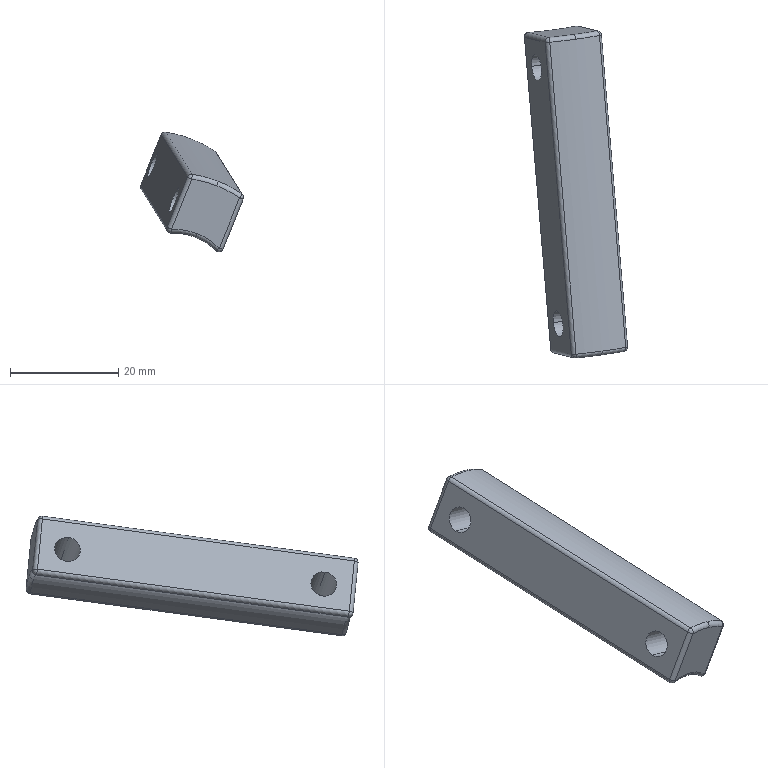Part | SolidWorks | features SplitBody 1 | 1 solid | 38 faces | box 19.087 x 61.426 x 22.135 mm | volume 7223 mm3 | cylinder 16 | sphere 10 | torus 8 | plane 4 | commonest cylinder face diameters 1.6 x10 4.8 x4 22.4 x1 44.8 x1
STEP:
#1=CARTESIAN_POINT('',(555.469,342.028,-348.256));
#2=VERTEX_POINT('',#1);
#3=CARTESIAN_POINT('',(554.431,342.001,-348.705));
#4=VERTEX_POINT('',#3);
#5=CARTESIAN_POINT('',(554.73,341.927,-347.967));
#6=DIRECTION('',(-0.08315,0.9876,0.1332));
#7=DIRECTION('',(-0.374,0.09296,-0.9228));
#8=AXIS2_PLACEMENT_3D('',#5,#6,#7);
#9=CIRCLE('',#8,0.8);
#10=EDGE_CURVE('',#2,#4,#9,.T.);
#11=ORIENTED_EDGE('',*,*,#10,.T.);
#12=CARTESIAN_POINT('',(554.663,342.717,-347.86));
#13=VERTEX_POINT('',#12);
#14=CARTESIAN_POINT('',(554.73,341.927,-347.967));
#15=DIRECTION('',(0.9237,0.1265,-0.3616));
#16=DIRECTION('',(-0.3646,0.,-0.9312));
#17=AXIS2_PLACEMENT_3D('',#14,#15,#16);
#18=CIRCLE('',#17,0.8);
#19=EDGE_CURVE('',#4,#13,#18,.T.);
#20=ORIENTED_EDGE('',*,*,#19,.T.);
#21=CARTESIAN_POINT('',(554.73,341.927,-347.967));
#22=DIRECTION('',(0.374,-0.09296,0.9228));
#23=DIRECTION('',(0.9237,0.1265,-0.3616));
#24=AXIS2_PLACEMENT_3D('',#21,#22,#23);
#25=CIRCLE('',#24,0.8);
#26=EDGE_CURVE('',#2,#13,#25,.T.);
#27=ORIENTED_EDGE('',*,*,#26,.F.);
#28=EDGE_LOOP('',(#11,#20,#27));
#29=FACE_OUTER_BOUND('',#28,.T.);
#30=CARTESIAN_POINT('',(554.73,341.927,-347.967));
#31=DIRECTION('',(-0.9237,-0.1265,0.3616));
#32=DIRECTION('',(-0.374,0.09296,-0.9228));
#33=AXIS2_PLACEMENT_3D('',#30,#31,#32);
#34=SPHERICAL_SURFACE('',#33,0.8);
#35=ADVANCED_FACE('',(#29),#34,.T.);
#36=CARTESIAN_POINT('',(554.195,341.124,-336.341));
#37=VERTEX_POINT('',#36);
#38=CARTESIAN_POINT('',(558.427,341.781,-338.576));
#39=VERTEX_POINT('',#38);
#40=CARTESIAN_POINT('',(546.116,343.132,-356.273));
#41=DIRECTION('',(-0.08315,0.9876,0.1332));
#42=DIRECTION('',(0.374,-0.09296,0.9228));
#43=AXIS2_PLACEMENT_3D('',#40,#41,#42);
#44=CIRCLE('',#43,21.6);
#45=EDGE_CURVE('',#37,#39,#44,.T.);
#46=ORIENTED_EDGE('',*,*,#45,.F.);
#47=CARTESIAN_POINT('',(554.561,340.259,-335.71));
#48=VERTEX_POINT('',#47);
#49=CARTESIAN_POINT('',(554.261,340.334,-336.448));
#50=DIRECTION('',(0.9237,0.1265,-0.3616));
#51=DIRECTION('',(-0.3646,0.,-0.9312));
#52=AXIS2_PLACEMENT_3D('',#49,#50,#51);
#53=CIRCLE('',#52,0.8);
#54=EDGE_CURVE('',#37,#48,#53,.T.);
#55=ORIENTED_EDGE('',*,*,#54,.T.);
#56=CARTESIAN_POINT('',(558.949,340.941,-338.027));
#57=VERTEX_POINT('',#56);
#58=CARTESIAN_POINT('',(546.183,342.342,-356.379));
#59=DIRECTION('',(0.08315,-0.9876,-0.1332));
#60=DIRECTION('',(0.374,-0.09296,0.9228));
#61=AXIS2_PLACEMENT_3D('',#58,#59,#60);
#62=CIRCLE('',#61,22.4);
#63=EDGE_CURVE('',#57,#48,#62,.T.);
#64=ORIENTED_EDGE('',*,*,#63,.F.);
#65=CARTESIAN_POINT('',(558.493,340.991,-338.682));
#66=DIRECTION('',(0.8175,0.144,-0.5577));
#67=DIRECTION('',(0.5699,-0.06252,0.8193));
#68=AXIS2_PLACEMENT_3D('',#65,#66,#67);
#69=CIRCLE('',#68,0.8);
#70=EDGE_CURVE('',#39,#57,#69,.T.);
#71=ORIENTED_EDGE('',*,*,#70,.F.);
#72=EDGE_LOOP('',(#46,#55,#64,#71));
#73=FACE_OUTER_BOUND('',#72,.T.);
#74=CARTESIAN_POINT('',(546.183,342.342,-356.379));
#75=DIRECTION('',(0.08315,-0.9876,-0.1332));
#76=DIRECTION('',(0.374,-0.09296,0.9228));
#77=AXIS2_PLACEMENT_3D('',#74,#75,#76);
#78=TOROIDAL_SURFACE('',#77,21.6,0.8);
#79=ADVANCED_FACE('',(#73),#78,.T.);
#80=CARTESIAN_POINT('',(560.325,284.352,-356.035));
#81=VERTEX_POINT('',#80);
#82=CARTESIAN_POINT('',(559.287,284.325,-356.484));
#83=VERTEX_POINT('',#82);
#84=CARTESIAN_POINT('',(559.586,284.251,-355.745));
#85=DIRECTION('',(-0.08315,0.9876,0.1332));
#86=DIRECTION('',(0.374,-0.09296,0.9228));
#87=AXIS2_PLACEMENT_3D('',#84,#85,#86);
#88=CIRCLE('',#87,0.8);
#89=EDGE_CURVE('',#81,#83,#88,.T.);
#90=ORIENTED_EDGE('',*,*,#89,.T.);
#91=CARTESIAN_POINT('',(559.353,283.535,-356.59));
#92=DIRECTION('',(-0.08315,0.9876,0.1332));
#93=VECTOR('',#92,1000.);
#94=LINE('',#91,#93);
#95=EDGE_CURVE('',#83,#4,#94,.T.);
#96=ORIENTED_EDGE('',*,*,#95,.T.);
#97=ORIENTED_EDGE('',*,*,#10,.F.);
#98=CARTESIAN_POINT('',(560.391,283.562,-356.141));
#99=DIRECTION('',(-0.08315,0.9876,0.1332));
#100=VECTOR('',#99,1000.);
#101=LINE('',#98,#100);
#102=EDGE_CURVE('',#81,#2,#101,.T.);
#103=ORIENTED_EDGE('',*,*,#102,.F.);
#104=EDGE_LOOP('',(#90,#96,#97,#103));
#105=FACE_OUTER_BOUND('',#104,.T.);
#106=CARTESIAN_POINT('',(559.653,283.461,-355.852));
#107=DIRECTION('',(-0.08315,0.9876,0.1332));
#108=DIRECTION('',(-0.374,0.09296,-0.9228));
#109=AXIS2_PLACEMENT_3D('',#106,#107,#108);
#110=CYLINDRICAL_SURFACE('',#109,0.8);
#111=ADVANCED_FACE('',(#105),#110,.T.);
#112=CARTESIAN_POINT('',(550.372,341.3,-346.044));
#113=VERTEX_POINT('',#112);
#114=CARTESIAN_POINT('',(554.16,341.954,-348.527));
#115=VERTEX_POINT('',#114);
#116=CARTESIAN_POINT('',(546.183,342.342,-356.379));
#117=DIRECTION('',(-0.08315,0.9876,0.1332));
#118=DIRECTION('',(0.374,-0.09296,0.9228));
#119=AXIS2_PLACEMENT_3D('',#116,#117,#118);
#120=CIRCLE('',#119,11.2);
#121=EDGE_CURVE('',#113,#115,#120,.T.);
#122=ORIENTED_EDGE('',*,*,#121,.F.);
#123=CARTESIAN_POINT('',(550.604,342.016,-345.2));
#124=VERTEX_POINT('',#123);
#125=CARTESIAN_POINT('',(550.671,341.226,-345.306));
#126=DIRECTION('',(0.9237,0.1265,-0.3616));
#127=DIRECTION('',(-0.3646,0.,-0.9312));
#128=AXIS2_PLACEMENT_3D('',#125,#126,#127);
#129=CIRCLE('',#128,0.8);
#130=EDGE_CURVE('',#113,#124,#129,.T.);
#131=ORIENTED_EDGE('',*,*,#130,.T.);
#132=CARTESIAN_POINT('',(546.116,343.132,-356.273));
#133=DIRECTION('',(0.08315,-0.9876,-0.1332));
#134=DIRECTION('',(0.374,-0.09296,0.9228));
#135=AXIS2_PLACEMENT_3D('',#132,#133,#134);
#136=CIRCLE('',#135,12.);
#137=EDGE_CURVE('',#13,#124,#136,.T.);
#138=ORIENTED_EDGE('',*,*,#137,.F.);
#139=CARTESIAN_POINT('',(554.73,341.927,-347.967));
#140=DIRECTION('',(0.697,0.1532,-0.7006));
#141=DIRECTION('',(0.7123,-0.03458,0.7011));
#142=AXIS2_PLACEMENT_3D('',#139,#140,#141);
#143=CIRCLE('',#142,0.8);
#144=EDGE_CURVE('',#115,#13,#143,.T.);
#145=ORIENTED_EDGE('',*,*,#144,.F.);
#146=EDGE_LOOP('',(#122,#131,#138,#145));
#147=FACE_OUTER_BOUND('',#146,.T.);
#148=CARTESIAN_POINT('',(546.183,342.342,-356.379));
#149=DIRECTION('',(0.08315,-0.9876,-0.1332));
#150=DIRECTION('',(0.374,-0.09296,0.9228));
#151=AXIS2_PLACEMENT_3D('',#148,#149,#150);
#152=TOROIDAL_SURFACE('',#151,12.,0.8);
#153=ADVANCED_FACE('',(#147),#152,.T.);
#154=CARTESIAN_POINT('',(545.884,340.82,-345.287));
#155=VERTEX_POINT('',#154);
#156=CARTESIAN_POINT('',(545.563,340.786,-345.233));
#157=VERTEX_POINT('',#156);
#158=CARTESIAN_POINT('',(545.863,340.712,-344.495));
#159=DIRECTION('',(-0.08315,0.9876,0.1332));
#160=DIRECTION('',(-0.374,0.09296,-0.9228));
#161=AXIS2_PLACEMENT_3D('',#158,#159,#160);
#162=CIRCLE('',#161,0.8);
#163=EDGE_CURVE('',#155,#157,#162,.T.);
#164=ORIENTED_EDGE('',*,*,#163,.T.);
#165=CARTESIAN_POINT('',(545.796,341.502,-344.388));
#166=VERTEX_POINT('',#165);
#167=CARTESIAN_POINT('',(545.863,340.712,-344.495));
#168=DIRECTION('',(0.9237,0.1265,-0.3616));
#169=DIRECTION('',(-0.3646,0.,-0.9312));
#170=AXIS2_PLACEMENT_3D('',#167,#168,#169);
#171=CIRCLE('',#170,0.8);
#172=EDGE_CURVE('',#157,#166,#171,.T.);
#173=ORIENTED_EDGE('',*,*,#172,.T.);
#174=CARTESIAN_POINT('',(545.863,340.712,-344.495));
#175=DIRECTION('',(0.9962,0.0788,0.03765));
#176=DIRECTION('',(0.02668,0.1358,-0.9904));
#177=AXIS2_PLACEMENT_3D('',#174,#175,#176);
#178=CIRCLE('',#177,0.8);
#179=EDGE_CURVE('',#155,#166,#178,.T.);
#180=ORIENTED_EDGE('',*,*,#179,.F.);
#181=EDGE_LOOP('',(#164,#173,#180));
#182=FACE_OUTER_BOUND('',#181,.T.);
#183=CARTESIAN_POINT('',(545.863,340.712,-344.495));
#184=DIRECTION('',(-0.9237,-0.1265,0.3616));
#185=DIRECTION('',(-0.374,0.09296,-0.9228));
#186=AXIS2_PLACEMENT_3D('',#183,#184,#185);
#187=SPHERICAL_SURFACE('',#186,0.8);
#188=ADVANCED_FACE('',(#182),#187,.T.);
#189=CARTESIAN_POINT('',(559.417,282.584,-343.488));
#190=VERTEX_POINT('',#189);
#191=CARTESIAN_POINT('',(563.805,283.266,-345.805));
#192=VERTEX_POINT('',#191);
#193=CARTESIAN_POINT('',(551.039,284.666,-364.158));
#194=DIRECTION('',(-0.08315,0.9876,0.1332));
#195=DIRECTION('',(0.374,-0.09296,0.9228));
#196=AXIS2_PLACEMENT_3D('',#193,#194,#195);
#197=CIRCLE('',#196,22.4);
#198=EDGE_CURVE('',#190,#192,#197,.T.);
#199=ORIENTED_EDGE('',*,*,#198,.F.);
#200=CARTESIAN_POINT('',(559.184,281.868,-344.333));
#201=VERTEX_POINT('',#200);
#202=CARTESIAN_POINT('',(559.118,282.658,-344.227));
#203=DIRECTION('',(0.9237,0.1265,-0.3616));
#204=DIRECTION('',(-0.3646,0.,-0.9312));
#205=AXIS2_PLACEMENT_3D('',#202,#203,#204);
#206=CIRCLE('',#205,0.8);
#207=EDGE_CURVE('',#190,#201,#206,.T.);
#208=ORIENTED_EDGE('',*,*,#207,.T.);
#209=CARTESIAN_POINT('',(563.416,282.526,-346.567));
#210=VERTEX_POINT('',#209);
#211=CARTESIAN_POINT('',(551.105,283.876,-364.265));
#212=DIRECTION('',(0.08315,-0.9876,-0.1332));
#213=DIRECTION('',(0.374,-0.09296,0.9228));
#214=AXIS2_PLACEMENT_3D('',#211,#212,#213);
#215=CIRCLE('',#214,21.6);
#216=EDGE_CURVE('',#210,#201,#215,.T.);
#217=ORIENTED_EDGE('',*,*,#216,.F.);
#218=CARTESIAN_POINT('',(563.349,283.316,-346.461));
#219=DIRECTION('',(0.8175,0.144,-0.5577));
#220=DIRECTION('',(0.5699,-0.06252,0.8193));
#221=AXIS2_PLACEMENT_3D('',#218,#219,#220);
#222=CIRCLE('',#221,0.8);
#223=EDGE_CURVE('',#192,#210,#222,.T.);
#224=ORIENTED_EDGE('',*,*,#223,.F.);
#225=EDGE_LOOP('',(#199,#208,#217,#224));
#226=FACE_OUTER_BOUND('',#225,.T.);
#227=CARTESIAN_POINT('',(551.039,284.666,-364.158));
#228=DIRECTION('',(0.08315,-0.9876,-0.1332));
#229=DIRECTION('',(0.374,-0.09296,0.9228));
#230=AXIS2_PLACEMENT_3D('',#227,#228,#229);
#231=TOROIDAL_SURFACE('',#230,21.6,0.8);
#232=ADVANCED_FACE('',(#226),#231,.T.);
#233=CARTESIAN_POINT('',(555.594,282.76,-353.192));
#234=VERTEX_POINT('',#233);
#235=CARTESIAN_POINT('',(559.653,283.461,-355.852));
#236=VERTEX_POINT('',#235);
#237=CARTESIAN_POINT('',(551.105,283.876,-364.265));
#238=DIRECTION('',(-0.08315,0.9876,0.1332));
#239=DIRECTION('',(0.374,-0.09296,0.9228));
#240=AXIS2_PLACEMENT_3D('',#237,#238,#239);
#241=CIRCLE('',#240,12.);
#242=EDGE_CURVE('',#234,#236,#241,.T.);
#243=ORIENTED_EDGE('',*,*,#242,.F.);
#244=CARTESIAN_POINT('',(555.228,283.625,-353.823));
#245=VERTEX_POINT('',#244);
#246=CARTESIAN_POINT('',(555.527,283.551,-353.085));
#247=DIRECTION('',(0.9237,0.1265,-0.3616));
#248=DIRECTION('',(-0.3646,0.,-0.9312));
#249=AXIS2_PLACEMENT_3D('',#246,#247,#248);
#250=CIRCLE('',#249,0.8);
#251=EDGE_CURVE('',#234,#245,#250,.T.);
#252=ORIENTED_EDGE('',*,*,#251,.T.);
#253=CARTESIAN_POINT('',(559.016,284.279,-356.306));
#254=VERTEX_POINT('',#253);
#255=CARTESIAN_POINT('',(551.039,284.666,-364.158));
#256=DIRECTION('',(0.08315,-0.9876,-0.1332));
#257=DIRECTION('',(0.374,-0.09296,0.9228));
#258=AXIS2_PLACEMENT_3D('',#255,#256,#257);
#259=CIRCLE('',#258,11.2);
#260=EDGE_CURVE('',#254,#245,#259,.T.);
#261=ORIENTED_EDGE('',*,*,#260,.F.);
#262=CARTESIAN_POINT('',(559.586,284.251,-355.745));
#263=DIRECTION('',(0.697,0.1532,-0.7006));
#264=DIRECTION('',(0.7123,-0.03458,0.7011));
#265=AXIS2_PLACEMENT_3D('',#262,#263,#264);
#266=CIRCLE('',#265,0.8);
#267=EDGE_CURVE('',#236,#254,#266,.T.);
#268=ORIENTED_EDGE('',*,*,#267,.F.);
#269=EDGE_LOOP('',(#243,#252,#261,#268));
#270=FACE_OUTER_BOUND('',#269,.T.);
#271=CARTESIAN_POINT('',(551.039,284.666,-364.158));
#272=DIRECTION('',(0.08315,-0.9876,-0.1332));
#273=DIRECTION('',(0.374,-0.09296,0.9228));
#274=AXIS2_PLACEMENT_3D('',#271,#272,#273);
#275=TOROIDAL_SURFACE('',#274,12.,0.8);
#276=ADVANCED_FACE('',(#270),#275,.T.);
#277=CARTESIAN_POINT('',(550.74,283.145,-353.066));
#278=VERTEX_POINT('',#277);
#279=CARTESIAN_POINT('',(550.419,283.111,-353.012));
#280=VERTEX_POINT('',#279);
#281=CARTESIAN_POINT('',(550.719,283.036,-352.274));
#282=DIRECTION('',(-0.08315,0.9876,0.1332));
#283=DIRECTION('',(0.374,-0.09296,0.9228));
#284=AXIS2_PLACEMENT_3D('',#281,#282,#283);
#285=CIRCLE('',#284,0.8);
#286=EDGE_CURVE('',#278,#280,#285,.T.);
#287=ORIENTED_EDGE('',*,*,#286,.T.);
#288=CARTESIAN_POINT('',(550.486,282.321,-353.118));
#289=DIRECTION('',(-0.08315,0.9876,0.1332));
#290=VECTOR('',#289,1000.);
#291=LINE('',#288,#290);
#292=EDGE_CURVE('',#280,#157,#291,.T.);
#293=ORIENTED_EDGE('',*,*,#292,.T.);
#294=ORIENTED_EDGE('',*,*,#163,.F.);
#295=CARTESIAN_POINT('',(550.806,282.355,-353.172));
#296=DIRECTION('',(-0.08315,0.9876,0.1332));
#297=VECTOR('',#296,1000.);
#298=LINE('',#295,#297);
#299=EDGE_CURVE('',#278,#155,#298,.T.);
#300=ORIENTED_EDGE('',*,*,#299,.F.);
#301=EDGE_LOOP('',(#287,#293,#294,#300));
#302=FACE_OUTER_BOUND('',#301,.T.);
#303=CARTESIAN_POINT('',(550.785,282.246,-352.38));
#304=DIRECTION('',(-0.08315,0.9876,0.1332));
#305=DIRECTION('',(-0.374,0.09296,-0.9228));
#306=AXIS2_PLACEMENT_3D('',#303,#304,#305);
#307=CYLINDRICAL_SURFACE('',#306,0.8);
#308=ADVANCED_FACE('',(#302),#307,.T.);
#309=CARTESIAN_POINT('',(562.547,288.828,-348.794));
#310=VERTEX_POINT('',#309);
#311=CARTESIAN_POINT('',(560.751,289.274,-353.224));
#312=VERTEX_POINT('',#311);
#313=CARTESIAN_POINT('',(561.649,289.051,-351.009));
#314=DIRECTION('',(-0.9237,-0.1265,0.3616));
#315=DIRECTION('',(-0.374,0.09296,-0.9228));
#316=AXIS2_PLACEMENT_3D('',#313,#314,#315);
#317=CIRCLE('',#316,2.4);
#318=EDGE_CURVE('',#310,#312,#317,.T.);
#319=ORIENTED_EDGE('',*,*,#318,.F.);
#320=CARTESIAN_POINT('',(552.201,287.411,-344.744));
#321=VERTEX_POINT('',#320);
#322=CARTESIAN_POINT('',(562.547,288.828,-348.794));
#323=DIRECTION('',(-0.9237,-0.1265,0.3616));
#324=VECTOR('',#323,1000.);
#325=LINE('',#322,#324);
#326=EDGE_CURVE('',#310,#321,#325,.T.);
#327=ORIENTED_EDGE('',*,*,#326,.T.);
#328=CARTESIAN_POINT('',(550.406,287.857,-349.173));
#329=VERTEX_POINT('',#328);
#330=CARTESIAN_POINT('',(551.304,287.634,-346.958));
#331=DIRECTION('',(-0.9237,-0.1265,0.3616));
#332=DIRECTION('',(-0.374,0.09296,-0.9228));
#333=AXIS2_PLACEMENT_3D('',#330,#331,#332);
#334=CIRCLE('',#333,2.4);
#335=EDGE_CURVE('',#321,#329,#334,.T.);
#336=ORIENTED_EDGE('',*,*,#335,.T.);
#337=CARTESIAN_POINT('',(560.751,289.274,-353.224));
#338=DIRECTION('',(-0.9237,-0.1265,0.3616));
#339=VECTOR('',#338,1000.);
#340=LINE('',#337,#339);
#341=EDGE_CURVE('',#312,#329,#340,.T.);
#342=ORIENTED_EDGE('',*,*,#341,.F.);
#343=EDGE_LOOP('',(#319,#327,#336,#342));
#344=FACE_OUTER_BOUND('',#343,.T.);
#345=CARTESIAN_POINT('',(561.649,289.051,-351.009));
#346=DIRECTION('',(-0.9237,-0.1265,0.3616));
#347=DIRECTION('',(-0.374,0.09296,-0.9228));
#348=AXIS2_PLACEMENT_3D('',#345,#346,#347);
#349=CYLINDRICAL_SURFACE('',#348,2.4);
#350=ADVANCED_FACE('',(#344),#349,.F.);
#351=CARTESIAN_POINT('',(558.555,336.233,-342.401));
#352=VERTEX_POINT('',#351);
#353=CARTESIAN_POINT('',(556.76,336.679,-346.83));
#354=VERTEX_POINT('',#353);
#355=CARTESIAN_POINT('',(557.658,336.456,-344.615));
#356=DIRECTION('',(-0.9237,-0.1265,0.3616));
#357=DIRECTION('',(-0.374,0.09296,-0.9228));
#358=AXIS2_PLACEMENT_3D('',#355,#356,#357);
#359=CIRCLE('',#358,2.4);
#360=EDGE_CURVE('',#352,#354,#359,.T.);
#361=ORIENTED_EDGE('',*,*,#360,.F.);
#362=CARTESIAN_POINT('',(548.21,334.815,-338.35));
#363=VERTEX_POINT('',#362);
#364=CARTESIAN_POINT('',(558.555,336.233,-342.401));
#365=DIRECTION('',(-0.9237,-0.1265,0.3616));
#366=VECTOR('',#365,1000.);
#367=LINE('',#364,#366);
#368=EDGE_CURVE('',#352,#363,#367,.T.);
#369=ORIENTED_EDGE('',*,*,#368,.T.);
#370=CARTESIAN_POINT('',(546.415,335.262,-342.78));
#371=VERTEX_POINT('',#370);
#372=CARTESIAN_POINT('',(547.312,335.038,-340.565));
#373=DIRECTION('',(-0.9237,-0.1265,0.3616));
#374=DIRECTION('',(-0.374,0.09296,-0.9228));
#375=AXIS2_PLACEMENT_3D('',#372,#373,#374);
#376=CIRCLE('',#375,2.4);
#377=EDGE_CURVE('',#363,#371,#376,.T.);
#378=ORIENTED_EDGE('',*,*,#377,.T.);
#379=CARTESIAN_POINT('',(556.76,336.679,-346.83));
#380=DIRECTION('',(-0.9237,-0.1265,0.3616));
#381=VECTOR('',#380,1000.);
#382=LINE('',#379,#381);
#383=EDGE_CURVE('',#354,#371,#382,.T.);
#384=ORIENTED_EDGE('',*,*,#383,.F.);
#385=EDGE_LOOP('',(#361,#369,#378,#384));
#386=FACE_OUTER_BOUND('',#385,.T.);
#387=CARTESIAN_POINT('',(557.658,336.456,-344.615));
#388=DIRECTION('',(-0.9237,-0.1265,0.3616));
#389=DIRECTION('',(-0.374,0.09296,-0.9228));
#390=AXIS2_PLACEMENT_3D('',#387,#388,#389);
#391=CYLINDRICAL_SURFACE('',#390,2.4);
#392=ADVANCED_FACE('',(#386),#391,.F.);
#393=ORIENTED_EDGE('',*,*,#299,.T.);
#394=CARTESIAN_POINT('',(546.183,342.342,-356.379));
#395=DIRECTION('',(-0.08315,0.9876,0.1332));
#396=DIRECTION('',(0.374,-0.09296,0.9228));
#397=AXIS2_PLACEMENT_3D('',#394,#395,#396);
#398=CIRCLE('',#397,11.2);
#399=EDGE_CURVE('',#155,#113,#398,.T.);
#400=ORIENTED_EDGE('',*,*,#399,.T.);
#401=ORIENTED_EDGE('',*,*,#121,.T.);
#402=CARTESIAN_POINT('',(559.083,283.489,-356.413));
#403=DIRECTION('',(0.08315,-0.9876,-0.1332));
#404=VECTOR('',#403,1000.);
#405=LINE('',#402,#404);
#406=EDGE_CURVE('',#115,#254,#405,.T.);
#407=ORIENTED_EDGE('',*,*,#406,.T.);
#408=ORIENTED_EDGE('',*,*,#260,.T.);
#409=CARTESIAN_POINT('',(551.039,284.666,-364.158));
#410=DIRECTION('',(0.08315,-0.9876,-0.1332));
#411=DIRECTION('',(0.374,-0.09296,0.9228));
#412=AXIS2_PLACEMENT_3D('',#409,#410,#411);
#413=CIRCLE('',#412,11.2);
#414=EDGE_CURVE('',#245,#278,#413,.T.);
#415=ORIENTED_EDGE('',*,*,#414,.T.);
#416=EDGE_LOOP('',(#393,#400,#401,#407,#408,#415));
#417=FACE_OUTER_BOUND('',#416,.T.);
#418=CARTESIAN_POINT('',(551.105,283.876,-364.265));
#419=DIRECTION('',(-0.08315,0.9876,0.1332));
#420=DIRECTION('',(-0.374,0.09296,-0.9228));
#421=AXIS2_PLACEMENT_3D('',#418,#419,#420);
#422=CYLINDRICAL_SURFACE('',#421,11.2);
#423=ADVANCED_FACE('',(#417),#422,.F.);
#424=ORIENTED_EDGE('',*,*,#102,.T.);
#425=CARTESIAN_POINT('',(559.232,341.093,-338.971));
#426=VERTEX_POINT('',#425);
#427=CARTESIAN_POINT('',(554.983,342.149,-349.454));
#428=DIRECTION('',(0.374,-0.09296,0.9228));
#429=VECTOR('',#428,1000.);
#430=LINE('',#427,#429);
#431=EDGE_CURVE('',#2,#426,#430,.T.);
#432=ORIENTED_EDGE('',*,*,#431,.T.);
#433=CARTESIAN_POINT('',(564.088,283.417,-346.75));
#434=VERTEX_POINT('',#433);
#435=CARTESIAN_POINT('',(564.155,282.627,-346.857));
#436=DIRECTION('',(0.08315,-0.9876,-0.1332));
#437=VECTOR('',#436,1000.);
#438=LINE('',#435,#437);
#439=EDGE_CURVE('',#426,#434,#438,.T.);
#440=ORIENTED_EDGE('',*,*,#439,.T.);
#441=CARTESIAN_POINT('',(559.839,284.473,-357.233));
#442=DIRECTION('',(-0.374,0.09296,-0.9228));
#443=VECTOR('',#442,1000.);
#444=LINE('',#441,#443);
#445=EDGE_CURVE('',#434,#81,#444,.T.);
#446=ORIENTED_EDGE('',*,*,#445,.T.);
#447=EDGE_LOOP('',(#424,#432,#440,#446));
#448=FACE_OUTER_BOUND('',#447,.T.);
#449=CARTESIAN_POINT('',(561.649,289.051,-351.009));
#450=DIRECTION('',(-0.9237,-0.1265,0.3616));
#451=DIRECTION('',(-0.374,0.09296,-0.9228));
#452=AXIS2_PLACEMENT_3D('',#449,#450,#451);
#453=CIRCLE('',#452,2.4);
#454=EDGE_CURVE('',#312,#310,#453,.T.);
#455=ORIENTED_EDGE('',*,*,#454,.T.);
#456=ORIENTED_EDGE('',*,*,#318,.T.);
#457=EDGE_LOOP('',(#455,#456));
#458=FACE_BOUND('',#457,.T.);
#459=CARTESIAN_POINT('',(557.658,336.456,-344.615));
#460=DIRECTION('',(-0.9237,-0.1265,0.3616));
#461=DIRECTION('',(-0.374,0.09296,-0.9228));
#462=AXIS2_PLACEMENT_3D('',#459,#460,#461);
#463=CIRCLE('',#462,2.4);
#464=EDGE_CURVE('',#354,#352,#463,.T.);
#465=ORIENTED_EDGE('',*,*,#464,.T.);
#466=ORIENTED_EDGE('',*,*,#360,.T.);
#467=EDGE_LOOP('',(#465,#466));
#468=FACE_BOUND('',#467,.T.);
#469=CARTESIAN_POINT('',(559.906,283.683,-357.34));
#470=DIRECTION('',(-0.9237,-0.1265,0.3616));
#471=DIRECTION('',(-0.374,0.09296,-0.9228));
#472=AXIS2_PLACEMENT_3D('',#469,#470,#471);
#473=PLANE('',#472);
#474=ADVANCED_FACE('',(#448,#458,#468),#473,.F.);
#475=CARTESIAN_POINT('',(563.872,282.476,-345.912));
#476=DIRECTION('',(-0.08315,0.9876,0.1332));
#477=VECTOR('',#476,1000.);
#478=LINE('',#475,#477);
#479=EDGE_CURVE('',#192,#57,#478,.T.);
#480=ORIENTED_EDGE('',*,*,#479,.T.);
#481=ORIENTED_EDGE('',*,*,#63,.T.);
#482=CARTESIAN_POINT('',(549.753,339.681,-334.426));
#483=VERTEX_POINT('',#482);
#484=CARTESIAN_POINT('',(546.183,342.342,-356.379));
#485=DIRECTION('',(0.08315,-0.9876,-0.1332));
#486=DIRECTION('',(0.374,-0.09296,0.9228));
#487=AXIS2_PLACEMENT_3D('',#484,#485,#486);
#488=CIRCLE('',#487,22.4);
#489=EDGE_CURVE('',#48,#483,#488,.T.);
#490=ORIENTED_EDGE('',*,*,#489,.T.);
#491=CARTESIAN_POINT('',(554.609,282.006,-342.205));
#492=VERTEX_POINT('',#491);
#493=CARTESIAN_POINT('',(554.676,281.216,-342.312));
#494=DIRECTION('',(0.08315,-0.9876,-0.1332));
#495=VECTOR('',#494,1000.);
#496=LINE('',#493,#495);
#497=EDGE_CURVE('',#483,#492,#496,.T.);
#498=ORIENTED_EDGE('',*,*,#497,.T.);
#499=CARTESIAN_POINT('',(551.039,284.666,-364.158));
#500=DIRECTION('',(-0.08315,0.9876,0.1332));
#501=DIRECTION('',(0.374,-0.09296,0.9228));
#502=AXIS2_PLACEMENT_3D('',#499,#500,#501);
#503=CIRCLE('',#502,22.4);
#504=EDGE_CURVE('',#492,#190,#503,.T.);
#505=ORIENTED_EDGE('',*,*,#504,.T.);
#506=ORIENTED_EDGE('',*,*,#198,.T.);
#507=EDGE_LOOP('',(#480,#481,#490,#498,#505,#506));
#508=FACE_OUTER_BOUND('',#507,.T.);
#509=CARTESIAN_POINT('',(551.105,283.876,-364.265));
#510=DIRECTION('',(-0.08315,0.9876,0.1332));
#511=DIRECTION('',(-0.374,0.09296,-0.9228));
#512=AXIS2_PLACEMENT_3D('',#509,#510,#511);
#513=CYLINDRICAL_SURFACE('',#512,22.4);
#514=ADVANCED_FACE('',(#508),#513,.T.);
#515=CARTESIAN_POINT('',(553.743,282.,-342.7));
#516=VERTEX_POINT('',#515);
#517=CARTESIAN_POINT('',(548.887,339.675,-334.921));
#518=VERTEX_POINT('',#517);
#519=CARTESIAN_POINT('',(553.809,281.21,-342.806));
#520=DIRECTION('',(-0.08315,0.9876,0.1332));
#521=VECTOR('',#520,1000.);
#522=LINE('',#519,#521);
#523=EDGE_CURVE('',#516,#518,#522,.T.);
#524=ORIENTED_EDGE('',*,*,#523,.T.);
#525=CARTESIAN_POINT('',(545.124,340.611,-344.205));
#526=VERTEX_POINT('',#525);
#527=CARTESIAN_POINT('',(549.122,339.617,-334.341));
#528=DIRECTION('',(-0.374,0.09296,-0.9228));
#529=VECTOR('',#528,1000.);
#530=LINE('',#527,#529);
#531=EDGE_CURVE('',#518,#526,#530,.T.);
#532=ORIENTED_EDGE('',*,*,#531,.T.);
#533=CARTESIAN_POINT('',(549.98,282.935,-351.984));
#534=VERTEX_POINT('',#533);
#535=CARTESIAN_POINT('',(550.046,282.145,-352.091));
#536=DIRECTION('',(0.08315,-0.9876,-0.1332));
#537=VECTOR('',#536,1000.);
#538=LINE('',#535,#537);
#539=EDGE_CURVE('',#526,#534,#538,.T.);
#540=ORIENTED_EDGE('',*,*,#539,.T.);
#541=CARTESIAN_POINT('',(553.978,281.941,-342.12));
#542=DIRECTION('',(0.374,-0.09296,0.9228));
#543=VECTOR('',#542,1000.);
#544=LINE('',#541,#543);
#545=EDGE_CURVE('',#534,#516,#544,.T.);
#546=ORIENTED_EDGE('',*,*,#545,.T.);
#547=EDGE_LOOP('',(#524,#532,#540,#546));
#548=FACE_OUTER_BOUND('',#547,.T.);
#549=CARTESIAN_POINT('',(551.304,287.634,-346.958));
#550=DIRECTION('',(-0.9237,-0.1265,0.3616));
#551=DIRECTION('',(-0.374,0.09296,-0.9228));
#552=AXIS2_PLACEMENT_3D('',#549,#550,#551);
#553=CIRCLE('',#552,2.4);
#554=EDGE_CURVE('',#329,#321,#553,.T.);
#555=ORIENTED_EDGE('',*,*,#554,.F.);
#556=ORIENTED_EDGE('',*,*,#335,.F.);
#557=EDGE_LOOP('',(#555,#556));
#558=FACE_BOUND('',#557,.T.);
#559=CARTESIAN_POINT('',(547.312,335.038,-340.565));
#560=DIRECTION('',(-0.9237,-0.1265,0.3616));
#561=DIRECTION('',(-0.374,0.09296,-0.9228));
#562=AXIS2_PLACEMENT_3D('',#559,#560,#561);
#563=CIRCLE('',#562,2.4);
#564=EDGE_CURVE('',#371,#363,#563,.T.);
#565=ORIENTED_EDGE('',*,*,#564,.F.);
#566=ORIENTED_EDGE('',*,*,#377,.F.);
#567=EDGE_LOOP('',(#565,#566));
#568=FACE_BOUND('',#567,.T.);
#569=CARTESIAN_POINT('',(554.045,281.151,-342.226));
#570=DIRECTION('',(0.9237,0.1265,-0.3616));
#571=DIRECTION('',(0.374,-0.09296,0.9228));
#572=AXIS2_PLACEMENT_3D('',#569,#570,#571);
#573=PLANE('',#572);
#574=ADVANCED_FACE('',(#548,#558,#568),#573,.F.);
#575=ORIENTED_EDGE('',*,*,#216,.T.);
#576=CARTESIAN_POINT('',(554.548,281.311,-343.096));
#577=VERTEX_POINT('',#576);
#578=CARTESIAN_POINT('',(551.105,283.876,-364.265));
#579=DIRECTION('',(0.08315,-0.9876,-0.1332));
#580=DIRECTION('',(0.374,-0.09296,0.9228));
#581=AXIS2_PLACEMENT_3D('',#578,#579,#580);
#582=CIRCLE('',#581,21.6);
#583=EDGE_CURVE('',#201,#577,#582,.T.);
#584=ORIENTED_EDGE('',*,*,#583,.T.);
#585=CARTESIAN_POINT('',(550.785,282.246,-352.38));
#586=VERTEX_POINT('',#585);
#587=CARTESIAN_POINT('',(550.299,282.367,-353.579));
#588=DIRECTION('',(-0.374,0.09296,-0.9228));
#589=VECTOR('',#588,1000.);
#590=LINE('',#587,#589);
#591=EDGE_CURVE('',#577,#586,#590,.T.);
#592=ORIENTED_EDGE('',*,*,#591,.T.);
#593=CARTESIAN_POINT('',(551.105,283.876,-364.265));
#594=DIRECTION('',(-0.08315,0.9876,0.1332));
#595=DIRECTION('',(0.374,-0.09296,0.9228));
#596=AXIS2_PLACEMENT_3D('',#593,#594,#595);
#597=CIRCLE('',#596,12.);
#598=EDGE_CURVE('',#586,#234,#597,.T.);
#599=ORIENTED_EDGE('',*,*,#598,.T.);
#600=ORIENTED_EDGE('',*,*,#242,.T.);
#601=CARTESIAN_POINT('',(563.651,282.467,-345.987));
#602=DIRECTION('',(0.374,-0.09296,0.9228));
#603=VECTOR('',#602,1000.);
#604=LINE('',#601,#603);
#605=EDGE_CURVE('',#236,#210,#604,.T.);
#606=ORIENTED_EDGE('',*,*,#605,.T.);
#607=EDGE_LOOP('',(#575,#584,#592,#599,#600,#606));
#608=FACE_OUTER_BOUND('',#607,.T.);
#609=CARTESIAN_POINT('',(551.105,283.876,-364.265));
#610=DIRECTION('',(0.08315,-0.9876,-0.1332));
#611=DIRECTION('',(0.374,-0.09296,0.9228));
#612=AXIS2_PLACEMENT_3D('',#609,#610,#611);
#613=PLANE('',#612);
#614=ADVANCED_FACE('',(#608),#613,.T.);
#615=CARTESIAN_POINT('',(549.559,340.566,-335.104));
#616=VERTEX_POINT('',#615);
#617=CARTESIAN_POINT('',(541.683,342.524,-354.537));
#618=DIRECTION('',(0.374,-0.09296,0.9228));
#619=VECTOR('',#618,1000.);
#620=LINE('',#617,#619);
#621=EDGE_CURVE('',#166,#616,#620,.T.);
#622=ORIENTED_EDGE('',*,*,#621,.T.);
#623=CARTESIAN_POINT('',(546.116,343.132,-356.273));
#624=DIRECTION('',(-0.08315,0.9876,0.1332));
#625=DIRECTION('',(0.374,-0.09296,0.9228));
#626=AXIS2_PLACEMENT_3D('',#623,#624,#625);
#627=CIRCLE('',#626,21.6);
#628=EDGE_CURVE('',#616,#37,#627,.T.);
#629=ORIENTED_EDGE('',*,*,#628,.T.);
#630=ORIENTED_EDGE('',*,*,#45,.T.);
#631=CARTESIAN_POINT('',(550.55,343.739,-358.009));
#632=DIRECTION('',(-0.374,0.09296,-0.9228));
#633=VECTOR('',#632,1000.);
#634=LINE('',#631,#633);
#635=EDGE_CURVE('',#39,#13,#634,.T.);
#636=ORIENTED_EDGE('',*,*,#635,.T.);
#637=ORIENTED_EDGE('',*,*,#137,.T.);
#638=CARTESIAN_POINT('',(546.116,343.132,-356.273));
#639=DIRECTION('',(0.08315,-0.9876,-0.1332));
#640=DIRECTION('',(0.374,-0.09296,0.9228));
#641=AXIS2_PLACEMENT_3D('',#638,#639,#640);
#642=CIRCLE('',#641,12.);
#643=EDGE_CURVE('',#124,#166,#642,.T.);
#644=ORIENTED_EDGE('',*,*,#643,.T.);
#645=EDGE_LOOP('',(#622,#629,#630,#636,#637,#644));
#646=FACE_OUTER_BOUND('',#645,.T.);
#647=CARTESIAN_POINT('',(546.116,343.132,-356.273));
#648=DIRECTION('',(0.08315,-0.9876,-0.1332));
#649=DIRECTION('',(0.374,-0.09296,0.9228));
#650=AXIS2_PLACEMENT_3D('',#647,#648,#649);
#651=PLANE('',#650);
#652=ADVANCED_FACE('',(#646),#651,.F.);
#653=ORIENTED_EDGE('',*,*,#368,.F.);
#654=ORIENTED_EDGE('',*,*,#464,.F.);
#655=ORIENTED_EDGE('',*,*,#383,.T.);
#656=ORIENTED_EDGE('',*,*,#564,.T.);
#657=EDGE_LOOP('',(#653,#654,#655,#656));
#658=FACE_OUTER_BOUND('',#657,.T.);
#659=CARTESIAN_POINT('',(557.658,336.456,-344.615));
#660=DIRECTION('',(-0.9237,-0.1265,0.3616));
#661=DIRECTION('',(-0.374,0.09296,-0.9228));
#662=AXIS2_PLACEMENT_3D('',#659,#660,#661);
#663=CYLINDRICAL_SURFACE('',#662,2.4);
#664=ADVANCED_FACE('',(#658),#663,.F.);
#665=ORIENTED_EDGE('',*,*,#326,.F.);
#666=ORIENTED_EDGE('',*,*,#454,.F.);
#667=ORIENTED_EDGE('',*,*,#341,.T.);
#668=ORIENTED_EDGE('',*,*,#554,.T.);
#669=EDGE_LOOP('',(#665,#666,#667,#668));
#670=FACE_OUTER_BOUND('',#669,.T.);
#671=CARTESIAN_POINT('',(561.649,289.051,-351.009));
#672=DIRECTION('',(-0.9237,-0.1265,0.3616));
#673=DIRECTION('',(-0.374,0.09296,-0.9228));
#674=AXIS2_PLACEMENT_3D('',#671,#672,#673);
#675=CYLINDRICAL_SURFACE('',#674,2.4);
#676=ADVANCED_FACE('',(#670),#675,.F.);
#677=CARTESIAN_POINT('',(550.719,283.036,-352.274));
#678=DIRECTION('',(-0.374,0.09296,-0.9228));
#679=DIRECTION('',(0.9237,0.1265,-0.3616));
#680=AXIS2_PLACEMENT_3D('',#677,#678,#679);
#681=CIRCLE('',#680,0.8);
#682=EDGE_CURVE('',#586,#534,#681,.T.);
#683=ORIENTED_EDGE('',*,*,#682,.F.);
#684=ORIENTED_EDGE('',*,*,#591,.F.);
#685=CARTESIAN_POINT('',(554.482,282.101,-342.989));
#686=DIRECTION('',(0.374,-0.09296,0.9228));
#687=DIRECTION('',(-0.08315,0.9876,0.1332));
#688=AXIS2_PLACEMENT_3D('',#685,#686,#687);
#689=CIRCLE('',#688,0.8);
#690=EDGE_CURVE('',#516,#577,#689,.T.);
#691=ORIENTED_EDGE('',*,*,#690,.F.);
#692=ORIENTED_EDGE('',*,*,#545,.F.);
#693=EDGE_LOOP('',(#683,#684,#691,#692));
#694=FACE_OUTER_BOUND('',#693,.T.);
#695=CARTESIAN_POINT('',(546.605,284.059,-362.422));
#696=DIRECTION('',(0.374,-0.09296,0.9228));
#697=DIRECTION('',(-0.9237,-0.1265,0.3616));
#698=AXIS2_PLACEMENT_3D('',#695,#696,#697);
#699=CYLINDRICAL_SURFACE('',#698,0.8);
#700=ADVANCED_FACE('',(#694),#699,.T.);
#701=CARTESIAN_POINT('',(550.719,283.036,-352.274));
#702=DIRECTION('',(0.9962,0.0788,0.03765));
#703=DIRECTION('',(0.02668,0.1358,-0.9904));
#704=AXIS2_PLACEMENT_3D('',#701,#702,#703);
#705=CIRCLE('',#704,0.8);
#706=EDGE_CURVE('',#586,#278,#705,.T.);
#707=ORIENTED_EDGE('',*,*,#706,.F.);
#708=ORIENTED_EDGE('',*,*,#682,.T.);
#709=CARTESIAN_POINT('',(550.719,283.036,-352.274));
#710=DIRECTION('',(-0.08315,0.9876,0.1332));
#711=DIRECTION('',(0.374,-0.09296,0.9228));
#712=AXIS2_PLACEMENT_3D('',#709,#710,#711);
#713=CIRCLE('',#712,0.8);
#714=EDGE_CURVE('',#280,#534,#713,.T.);
#715=ORIENTED_EDGE('',*,*,#714,.F.);
#716=ORIENTED_EDGE('',*,*,#286,.F.);
#717=EDGE_LOOP('',(#707,#708,#715,#716));
#718=FACE_OUTER_BOUND('',#717,.T.);
#719=CARTESIAN_POINT('',(550.719,283.036,-352.274));
#720=DIRECTION('',(-0.9237,-0.1265,0.3616));
#721=DIRECTION('',(0.374,-0.09296,0.9228));
#722=AXIS2_PLACEMENT_3D('',#719,#720,#721);
#723=SPHERICAL_SURFACE('',#722,0.8);
#724=ADVANCED_FACE('',(#718),#723,.T.);
#725=CARTESIAN_POINT('',(554.482,282.101,-342.989));
#726=DIRECTION('',(-0.08315,0.9876,0.1332));
#727=DIRECTION('',(0.374,-0.09296,0.9228));
#728=AXIS2_PLACEMENT_3D('',#725,#726,#727);
#729=CIRCLE('',#728,0.8);
#730=EDGE_CURVE('',#516,#492,#729,.T.);
#731=ORIENTED_EDGE('',*,*,#730,.F.);
#732=ORIENTED_EDGE('',*,*,#690,.T.);
#733=CARTESIAN_POINT('',(554.482,282.101,-342.989));
#734=DIRECTION('',(0.9837,0.1027,-0.1475));
#735=DIRECTION('',(-0.1594,0.1188,-0.98));
#736=AXIS2_PLACEMENT_3D('',#733,#734,#735);
#737=CIRCLE('',#736,0.8);
#738=EDGE_CURVE('',#492,#577,#737,.T.);
#739=ORIENTED_EDGE('',*,*,#738,.F.);
#740=EDGE_LOOP('',(#731,#732,#739));
#741=FACE_OUTER_BOUND('',#740,.T.);
#742=CARTESIAN_POINT('',(554.482,282.101,-342.989));
#743=DIRECTION('',(-0.9237,-0.1265,0.3616));
#744=DIRECTION('',(0.374,-0.09296,0.9228));
#745=AXIS2_PLACEMENT_3D('',#742,#743,#744);
#746=SPHERICAL_SURFACE('',#745,0.8);
#747=ADVANCED_FACE('',(#741),#746,.T.);
#748=ORIENTED_EDGE('',*,*,#292,.F.);
#749=ORIENTED_EDGE('',*,*,#714,.T.);
#750=ORIENTED_EDGE('',*,*,#539,.F.);
#751=CARTESIAN_POINT('',(545.863,340.712,-344.495));
#752=DIRECTION('',(-0.08315,0.9876,0.1332));
#753=DIRECTION('',(-0.374,0.09296,-0.9228));
#754=AXIS2_PLACEMENT_3D('',#751,#752,#753);
#755=CIRCLE('',#754,0.8);
#756=EDGE_CURVE('',#157,#526,#755,.T.);
#757=ORIENTED_EDGE('',*,*,#756,.F.);
#758=EDGE_LOOP('',(#748,#749,#750,#757));
#759=FACE_OUTER_BOUND('',#758,.T.);
#760=CARTESIAN_POINT('',(550.785,282.246,-352.38));
#761=DIRECTION('',(-0.08315,0.9876,0.1332));
#762=DIRECTION('',(-0.374,0.09296,-0.9228));
#763=AXIS2_PLACEMENT_3D('',#760,#761,#762);
#764=CYLINDRICAL_SURFACE('',#763,0.8);
#765=ADVANCED_FACE('',(#759),#764,.T.);
#766=ORIENTED_EDGE('',*,*,#251,.F.);
#767=ORIENTED_EDGE('',*,*,#598,.F.);
#768=ORIENTED_EDGE('',*,*,#706,.T.);
#769=ORIENTED_EDGE('',*,*,#414,.F.);
#770=EDGE_LOOP('',(#766,#767,#768,#769));
#771=FACE_OUTER_BOUND('',#770,.T.);
#772=CARTESIAN_POINT('',(551.039,284.666,-364.158));
#773=DIRECTION('',(0.08315,-0.9876,-0.1332));
#774=DIRECTION('',(0.374,-0.09296,0.9228));
#775=AXIS2_PLACEMENT_3D('',#772,#773,#774);
#776=TOROIDAL_SURFACE('',#775,12.,0.8);
#777=ADVANCED_FACE('',(#771),#776,.T.);
#778=CARTESIAN_POINT('',(563.349,283.316,-346.461));
#779=DIRECTION('',(0.374,-0.09296,0.9228));
#780=DIRECTION('',(-0.9237,-0.1265,0.3616));
#781=AXIS2_PLACEMENT_3D('',#778,#779,#780);
#782=CIRCLE('',#781,0.8);
#783=EDGE_CURVE('',#210,#434,#782,.T.);
#784=ORIENTED_EDGE('',*,*,#783,.F.);
#785=ORIENTED_EDGE('',*,*,#605,.F.);
#786=CARTESIAN_POINT('',(559.586,284.251,-355.745));
#787=DIRECTION('',(-0.374,0.09296,-0.9228));
#788=DIRECTION('',(0.9237,0.1265,-0.3616));
#789=AXIS2_PLACEMENT_3D('',#786,#787,#788);
#790=CIRCLE('',#789,0.8);
#791=EDGE_CURVE('',#81,#236,#790,.T.);
#792=ORIENTED_EDGE('',*,*,#791,.F.);
#793=ORIENTED_EDGE('',*,*,#445,.F.);
#794=EDGE_LOOP('',(#784,#785,#792,#793));
#795=FACE_OUTER_BOUND('',#794,.T.);
#796=CARTESIAN_POINT('',(555.473,285.273,-365.894));
#797=DIRECTION('',(-0.374,0.09296,-0.9228));
#798=DIRECTION('',(0.9237,0.1265,-0.3616));
#799=AXIS2_PLACEMENT_3D('',#796,#797,#798);
#800=CYLINDRICAL_SURFACE('',#799,0.8);
#801=ADVANCED_FACE('',(#795),#800,.T.);
#802=ORIENTED_EDGE('',*,*,#207,.F.);
#803=ORIENTED_EDGE('',*,*,#504,.F.);
#804=ORIENTED_EDGE('',*,*,#738,.T.);
#805=ORIENTED_EDGE('',*,*,#583,.F.);
#806=EDGE_LOOP('',(#802,#803,#804,#805));
#807=FACE_OUTER_BOUND('',#806,.T.);
#808=CARTESIAN_POINT('',(551.039,284.666,-364.158));
#809=DIRECTION('',(0.08315,-0.9876,-0.1332));
#810=DIRECTION('',(0.374,-0.09296,0.9228));
#811=AXIS2_PLACEMENT_3D('',#808,#809,#810);
#812=TOROIDAL_SURFACE('',#811,21.6,0.8);
#813=ADVANCED_FACE('',(#807),#812,.T.);
#814=ORIENTED_EDGE('',*,*,#730,.T.);
#815=ORIENTED_EDGE('',*,*,#497,.F.);
#816=CARTESIAN_POINT('',(549.626,339.776,-335.21));
#817=DIRECTION('',(-0.08315,0.9876,0.1332));
#818=DIRECTION('',(-0.374,0.09296,-0.9228));
#819=AXIS2_PLACEMENT_3D('',#816,#817,#818);
#820=CIRCLE('',#819,0.8);
#821=EDGE_CURVE('',#518,#483,#820,.T.);
#822=ORIENTED_EDGE('',*,*,#821,.F.);
#823=ORIENTED_EDGE('',*,*,#523,.F.);
#824=EDGE_LOOP('',(#814,#815,#822,#823));
#825=FACE_OUTER_BOUND('',#824,.T.);
#826=CARTESIAN_POINT('',(554.548,281.311,-343.096));
#827=DIRECTION('',(-0.08315,0.9876,0.1332));
#828=DIRECTION('',(-0.374,0.09296,-0.9228));
#829=AXIS2_PLACEMENT_3D('',#826,#827,#828);
#830=CYLINDRICAL_SURFACE('',#829,0.8);
#831=ADVANCED_FACE('',(#825),#830,.T.);
#832=CARTESIAN_POINT('',(545.863,340.712,-344.495));
#833=DIRECTION('',(-0.374,0.09296,-0.9228));
#834=DIRECTION('',(0.9237,0.1265,-0.3616));
#835=AXIS2_PLACEMENT_3D('',#832,#833,#834);
#836=CIRCLE('',#835,0.8);
#837=EDGE_CURVE('',#526,#166,#836,.T.);
#838=ORIENTED_EDGE('',*,*,#837,.F.);
#839=ORIENTED_EDGE('',*,*,#531,.F.);
#840=CARTESIAN_POINT('',(549.626,339.776,-335.21));
#841=DIRECTION('',(0.374,-0.09296,0.9228));
#842=DIRECTION('',(-0.9237,-0.1265,0.3616));
#843=AXIS2_PLACEMENT_3D('',#840,#841,#842);
#844=CIRCLE('',#843,0.8);
#845=EDGE_CURVE('',#616,#518,#844,.T.);
#846=ORIENTED_EDGE('',*,*,#845,.F.);
#847=ORIENTED_EDGE('',*,*,#621,.F.);
#848=EDGE_LOOP('',(#838,#839,#846,#847));
#849=FACE_OUTER_BOUND('',#848,.T.);
#850=CARTESIAN_POINT('',(549.861,339.718,-334.63));
#851=DIRECTION('',(-0.374,0.09296,-0.9228));
#852=DIRECTION('',(0.9237,0.1265,-0.3616));
#853=AXIS2_PLACEMENT_3D('',#850,#851,#852);
#854=CYLINDRICAL_SURFACE('',#853,0.8);
#855=ADVANCED_FACE('',(#849),#854,.T.);
#856=ORIENTED_EDGE('',*,*,#172,.F.);
#857=ORIENTED_EDGE('',*,*,#756,.T.);
#858=ORIENTED_EDGE('',*,*,#837,.T.);
#859=EDGE_LOOP('',(#856,#857,#858));
#860=FACE_OUTER_BOUND('',#859,.T.);
#861=CARTESIAN_POINT('',(545.863,340.712,-344.495));
#862=DIRECTION('',(-0.9237,-0.1265,0.3616));
#863=DIRECTION('',(-0.374,0.09296,-0.9228));
#864=AXIS2_PLACEMENT_3D('',#861,#862,#863);
#865=SPHERICAL_SURFACE('',#864,0.8);
#866=ADVANCED_FACE('',(#860),#865,.T.);
#867=ORIENTED_EDGE('',*,*,#791,.T.);
#868=ORIENTED_EDGE('',*,*,#267,.T.);
#869=CARTESIAN_POINT('',(559.586,284.251,-355.745));
#870=DIRECTION('',(-0.08315,0.9876,0.1332));
#871=DIRECTION('',(0.374,-0.09296,0.9228));
#872=AXIS2_PLACEMENT_3D('',#869,#870,#871);
#873=CIRCLE('',#872,0.8);
#874=EDGE_CURVE('',#83,#254,#873,.T.);
#875=ORIENTED_EDGE('',*,*,#874,.F.);
#876=ORIENTED_EDGE('',*,*,#89,.F.);
#877=EDGE_LOOP('',(#867,#868,#875,#876));
#878=FACE_OUTER_BOUND('',#877,.T.);
#879=CARTESIAN_POINT('',(559.586,284.251,-355.745));
#880=DIRECTION('',(-0.9237,-0.1265,0.3616));
#881=DIRECTION('',(0.374,-0.09296,0.9228));
#882=AXIS2_PLACEMENT_3D('',#879,#880,#881);
#883=SPHERICAL_SURFACE('',#882,0.8);
#884=ADVANCED_FACE('',(#878),#883,.T.);
#885=ORIENTED_EDGE('',*,*,#223,.T.);
#886=ORIENTED_EDGE('',*,*,#783,.T.);
#887=CARTESIAN_POINT('',(563.349,283.316,-346.461));
#888=DIRECTION('',(-0.08315,0.9876,0.1332));
#889=DIRECTION('',(0.374,-0.09296,0.9228));
#890=AXIS2_PLACEMENT_3D('',#887,#888,#889);
#891=CIRCLE('',#890,0.8);
#892=EDGE_CURVE('',#192,#434,#891,.T.);
#893=ORIENTED_EDGE('',*,*,#892,.F.);
#894=EDGE_LOOP('',(#885,#886,#893));
#895=FACE_OUTER_BOUND('',#894,.T.);
#896=CARTESIAN_POINT('',(563.349,283.316,-346.461));
#897=DIRECTION('',(-0.9237,-0.1265,0.3616));
#898=DIRECTION('',(0.374,-0.09296,0.9228));
#899=AXIS2_PLACEMENT_3D('',#896,#897,#898);
#900=SPHERICAL_SURFACE('',#899,0.8);
#901=ADVANCED_FACE('',(#895),#900,.T.);
#902=ORIENTED_EDGE('',*,*,#845,.T.);
#903=ORIENTED_EDGE('',*,*,#821,.T.);
#904=CARTESIAN_POINT('',(549.626,339.776,-335.21));
#905=DIRECTION('',(0.9837,0.1027,-0.1475));
#906=DIRECTION('',(-0.1594,0.1188,-0.98));
#907=AXIS2_PLACEMENT_3D('',#904,#905,#906);
#908=CIRCLE('',#907,0.8);
#909=EDGE_CURVE('',#616,#483,#908,.T.);
#910=ORIENTED_EDGE('',*,*,#909,.F.);
#911=EDGE_LOOP('',(#902,#903,#910));
#912=FACE_OUTER_BOUND('',#911,.T.);
#913=CARTESIAN_POINT('',(549.626,339.776,-335.21));
#914=DIRECTION('',(-0.9237,-0.1265,0.3616));
#915=DIRECTION('',(-0.374,0.09296,-0.9228));
#916=AXIS2_PLACEMENT_3D('',#913,#914,#915);
#917=SPHERICAL_SURFACE('',#916,0.8);
#918=ADVANCED_FACE('',(#912),#917,.T.);
#919=ORIENTED_EDGE('',*,*,#130,.F.);
#920=ORIENTED_EDGE('',*,*,#399,.F.);
#921=ORIENTED_EDGE('',*,*,#179,.T.);
#922=ORIENTED_EDGE('',*,*,#643,.F.);
#923=EDGE_LOOP('',(#919,#920,#921,#922));
#924=FACE_OUTER_BOUND('',#923,.T.);
#925=CARTESIAN_POINT('',(546.183,342.342,-356.379));
#926=DIRECTION('',(0.08315,-0.9876,-0.1332));
#927=DIRECTION('',(0.374,-0.09296,0.9228));
#928=AXIS2_PLACEMENT_3D('',#925,#926,#927);
#929=TOROIDAL_SURFACE('',#928,12.,0.8);
#930=ADVANCED_FACE('',(#924),#929,.T.);
#931=ORIENTED_EDGE('',*,*,#95,.F.);
#932=ORIENTED_EDGE('',*,*,#874,.T.);
#933=ORIENTED_EDGE('',*,*,#406,.F.);
#934=CARTESIAN_POINT('',(554.73,341.927,-347.967));
#935=DIRECTION('',(-0.08315,0.9876,0.1332));
#936=DIRECTION('',(-0.374,0.09296,-0.9228));
#937=AXIS2_PLACEMENT_3D('',#934,#935,#936);
#938=CIRCLE('',#937,0.8);
#939=EDGE_CURVE('',#4,#115,#938,.T.);
#940=ORIENTED_EDGE('',*,*,#939,.F.);
#941=EDGE_LOOP('',(#931,#932,#933,#940));
#942=FACE_OUTER_BOUND('',#941,.T.);
#943=CARTESIAN_POINT('',(559.653,283.461,-355.852));
#944=DIRECTION('',(-0.08315,0.9876,0.1332));
#945=DIRECTION('',(-0.374,0.09296,-0.9228));
#946=AXIS2_PLACEMENT_3D('',#943,#944,#945);
#947=CYLINDRICAL_SURFACE('',#946,0.8);
#948=ADVANCED_FACE('',(#942),#947,.T.);
#949=ORIENTED_EDGE('',*,*,#892,.T.);
#950=ORIENTED_EDGE('',*,*,#439,.F.);
#951=CARTESIAN_POINT('',(558.493,340.991,-338.682));
#952=DIRECTION('',(-0.08315,0.9876,0.1332));
#953=DIRECTION('',(-0.374,0.09296,-0.9228));
#954=AXIS2_PLACEMENT_3D('',#951,#952,#953);
#955=CIRCLE('',#954,0.8);
#956=EDGE_CURVE('',#57,#426,#955,.T.);
#957=ORIENTED_EDGE('',*,*,#956,.F.);
#958=ORIENTED_EDGE('',*,*,#479,.F.);
#959=EDGE_LOOP('',(#949,#950,#957,#958));
#960=FACE_OUTER_BOUND('',#959,.T.);
#961=CARTESIAN_POINT('',(563.416,282.526,-346.567));
#962=DIRECTION('',(-0.08315,0.9876,0.1332));
#963=DIRECTION('',(-0.374,0.09296,-0.9228));
#964=AXIS2_PLACEMENT_3D('',#961,#962,#963);
#965=CYLINDRICAL_SURFACE('',#964,0.8);
#966=ADVANCED_FACE('',(#960),#965,.T.);
#967=ORIENTED_EDGE('',*,*,#54,.F.);
#968=ORIENTED_EDGE('',*,*,#628,.F.);
#969=ORIENTED_EDGE('',*,*,#909,.T.);
#970=ORIENTED_EDGE('',*,*,#489,.F.);
#971=EDGE_LOOP('',(#967,#968,#969,#970));
#972=FACE_OUTER_BOUND('',#971,.T.);
#973=CARTESIAN_POINT('',(546.183,342.342,-356.379));
#974=DIRECTION('',(0.08315,-0.9876,-0.1332));
#975=DIRECTION('',(0.374,-0.09296,0.9228));
#976=AXIS2_PLACEMENT_3D('',#973,#974,#975);
#977=TOROIDAL_SURFACE('',#976,21.6,0.8);
#978=ADVANCED_FACE('',(#972),#977,.T.);
#979=ORIENTED_EDGE('',*,*,#19,.F.);
#980=ORIENTED_EDGE('',*,*,#939,.T.);
#981=ORIENTED_EDGE('',*,*,#144,.T.);
#982=EDGE_LOOP('',(#979,#980,#981));
#983=FACE_OUTER_BOUND('',#982,.T.);
#984=CARTESIAN_POINT('',(554.73,341.927,-347.967));
#985=DIRECTION('',(-0.9237,-0.1265,0.3616));
#986=DIRECTION('',(-0.374,0.09296,-0.9228));
#987=AXIS2_PLACEMENT_3D('',#984,#985,#986);
#988=SPHERICAL_SURFACE('',#987,0.8);
#989=ADVANCED_FACE('',(#983),#988,.T.);
#990=ORIENTED_EDGE('',*,*,#70,.T.);
#991=ORIENTED_EDGE('',*,*,#956,.T.);
#992=CARTESIAN_POINT('',(558.493,340.991,-338.682));
#993=DIRECTION('',(-0.374,0.09296,-0.9228));
#994=DIRECTION('',(-0.08315,0.9876,0.1332));
#995=AXIS2_PLACEMENT_3D('',#992,#993,#994);
#996=CIRCLE('',#995,0.8);
#997=EDGE_CURVE('',#39,#426,#996,.T.);
#998=ORIENTED_EDGE('',*,*,#997,.F.);
#999=EDGE_LOOP('',(#990,#991,#998));
#1000=FACE_OUTER_BOUND('',#999,.T.);
#1001=CARTESIAN_POINT('',(558.493,340.991,-338.682));
#1002=DIRECTION('',(-0.9237,-0.1265,0.3616));
#1003=DIRECTION('',(-0.374,0.09296,-0.9228));
#1004=AXIS2_PLACEMENT_3D('',#1001,#1002,#1003);
#1005=SPHERICAL_SURFACE('',#1004,0.8);
#1006=ADVANCED_FACE('',(#1000),#1005,.T.);
#1007=ORIENTED_EDGE('',*,*,#26,.T.);
#1008=ORIENTED_EDGE('',*,*,#635,.F.);
#1009=ORIENTED_EDGE('',*,*,#997,.T.);
#1010=ORIENTED_EDGE('',*,*,#431,.F.);
#1011=EDGE_LOOP('',(#1007,#1008,#1009,#1010));
#1012=FACE_OUTER_BOUND('',#1011,.T.);
#1013=CARTESIAN_POINT('',(554.244,342.047,-349.165));
#1014=DIRECTION('',(0.374,-0.09296,0.9228));
#1015=DIRECTION('',(-0.9237,-0.1265,0.3616));
#1016=AXIS2_PLACEMENT_3D('',#1013,#1014,#1015);
#1017=CYLINDRICAL_SURFACE('',#1016,0.8);
#1018=ADVANCED_FACE('',(#1012),#1017,.T.);
#1019=CLOSED_SHELL('',(#35,#79,#111,#153,#188,#232,#276,#308,#350,#392,#423,#474,#514,#574,#614,#652,#664,#676,#700,#724,#747,#765,#777,#801,#813,#831,#855,#866,#884,#901,#918,#930,#948,#966,#978,#989,#1006,#1018));
#1020=MANIFOLD_SOLID_BREP('',#1019);
#1021=CARTESIAN_POINT('',(0.,0.,0.));
#1022=DIRECTION('',(0.,0.,1.));
#1023=DIRECTION('',(1.,0.,0.));
#1024=AXIS2_PLACEMENT_3D('',#1021,#1022,#1023);
#1025=(LENGTH_UNIT()NAMED_UNIT(*)SI_UNIT(.MILLI.,.METRE.));
#1026=UNCERTAINTY_MEASURE_WITH_UNIT(LENGTH_MEASURE(0.00001),#1025,'','');
#1027=(NAMED_UNIT(*)PLANE_ANGLE_UNIT()SI_UNIT($,.RADIAN.));
#1028=(NAMED_UNIT(*)SI_UNIT($,.STERADIAN.)SOLID_ANGLE_UNIT());
#1029=(GEOMETRIC_REPRESENTATION_CONTEXT(3)GLOBAL_UNCERTAINTY_ASSIGNED_CONTEXT((#1026))GLOBAL_UNIT_ASSIGNED_CONTEXT((#1025,#1027,#1028))REPRESENTATION_CONTEXT('',''));
#1030=ADVANCED_BREP_SHAPE_REPRESENTATION('',(#1020,#1024),#1029);